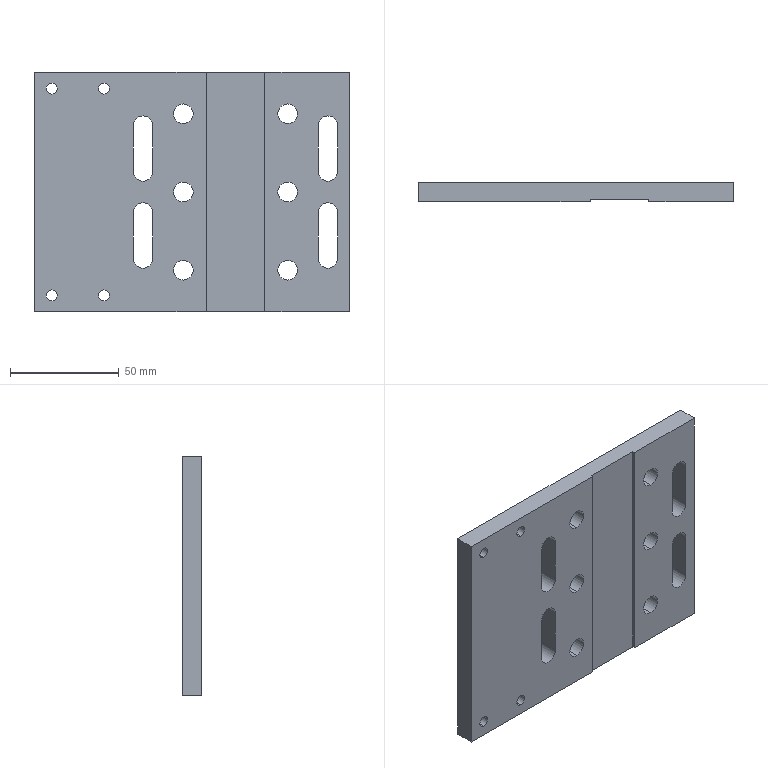Part | STEP file | 0245_207_Plate | 1 solid | 50 faces | box 145 x 9 x 110 mm | volume 127344 mm3 | cylinder 32 | plane 18 | commonest cylinder face diameters 9 x24 5 x8